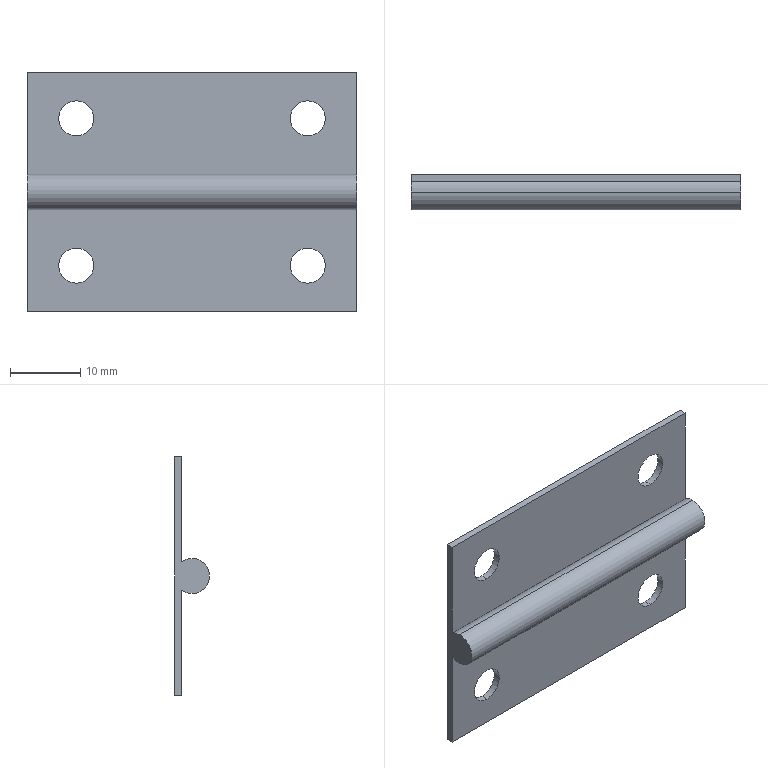Part | STEP file | 50 hinge | 1 solid | 18 faces | box 47 x 5 x 34 mm | volume 2311 mm3 | cylinder 11 | plane 7 | commonest cylinder face diameters 5 x11